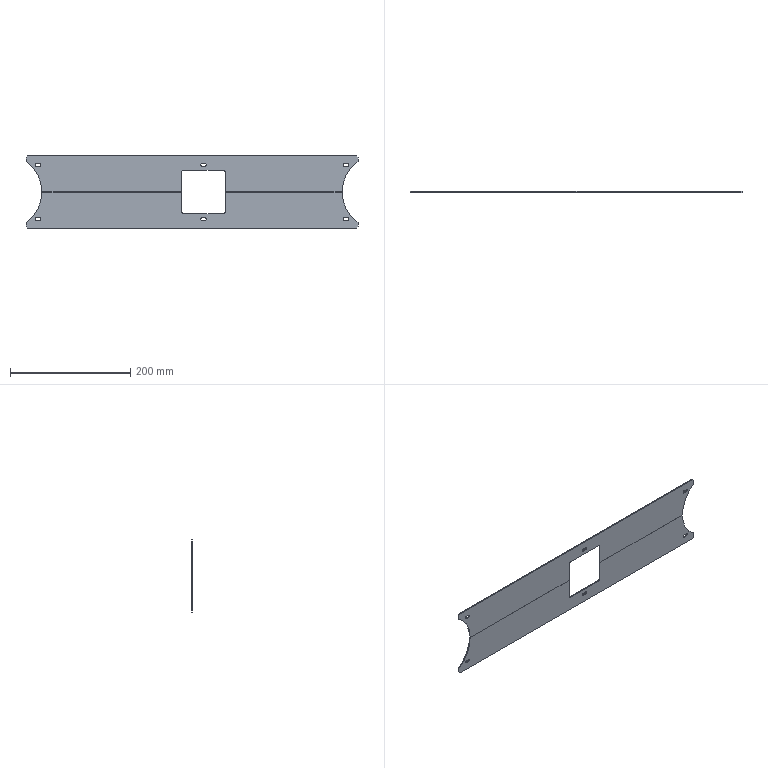Part | SolidWorks | features ICE 5, Chamfer 2, Extrusion 1, MirrorPattern 1 | 2 solids | 56 faces | box 552 x 1.5 x 120 mm | volume 85515 mm3 | plane 36 | cylinder 20 | commonest cylinder face diameters 4.5 x12 6 x4 123 x4